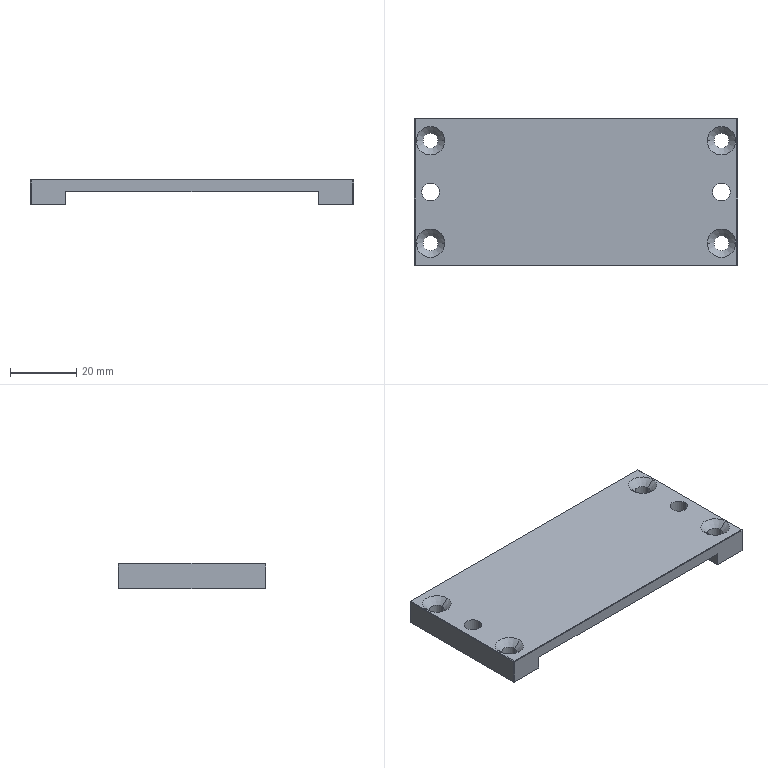Part | STEP file | 1 solid | 38 faces | box 97.7 x 44.7 x 7.7 mm | volume 18958 mm3 | plane 18 | cylinder 12 | cone 8 | commonest cylinder face diameters 4.5 x8 5.3 x4